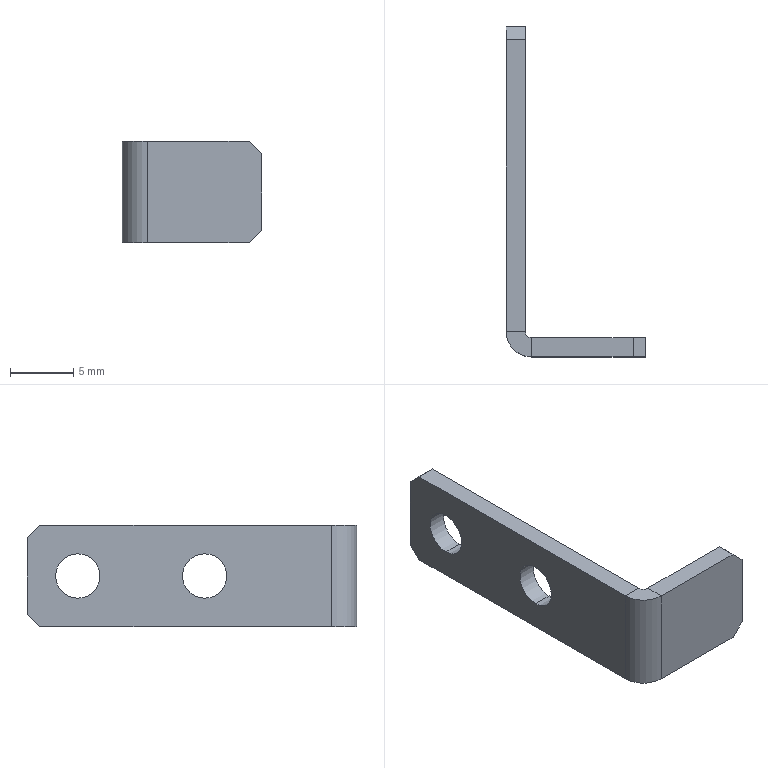Part | SolidWorks | features Chamfer 1, FlatPattern 1, HoleWzd 1, SMBaseFlange 1, SheetMetal 1 | 1 solid | 22 faces | box 11 x 26 x 8 mm | volume 387.699 mm3 | plane 16 | cylinder 6 | commonest cylinder face diameters 3.5 x4 1 x1 4 x1
STEP:
#1=CARTESIAN_POINT('',(1.5,22.,5.75));
#2=VERTEX_POINT('',#1);
#3=CARTESIAN_POINT('',(1.5,22.,2.25));
#4=VERTEX_POINT('',#3);
#5=CARTESIAN_POINT('',(1.5,22.,4.));
#6=DIRECTION('',(1.,0.,0.));
#7=DIRECTION('',(0.,1.,0.));
#8=AXIS2_PLACEMENT_3D('',#5,#6,#7);
#9=CIRCLE('',#8,1.75);
#10=EDGE_CURVE('',#2,#4,#9,.T.);
#11=ORIENTED_EDGE('',*,*,#10,.T.);
#12=CARTESIAN_POINT('',(0.,22.,2.25));
#13=VERTEX_POINT('',#12);
#14=CARTESIAN_POINT('',(0.,22.,2.25));
#15=DIRECTION('',(-1.,0.,0.));
#16=VECTOR('',#15,1000.);
#17=LINE('',#14,#16);
#18=EDGE_CURVE('',#4,#13,#17,.T.);
#19=ORIENTED_EDGE('',*,*,#18,.T.);
#20=CARTESIAN_POINT('',(0.,22.,5.75));
#21=VERTEX_POINT('',#20);
#22=CARTESIAN_POINT('',(0.,22.,4.));
#23=DIRECTION('',(-1.,0.,0.));
#24=DIRECTION('',(0.,0.,1.));
#25=AXIS2_PLACEMENT_3D('',#22,#23,#24);
#26=CIRCLE('',#25,1.75);
#27=EDGE_CURVE('',#13,#21,#26,.T.);
#28=ORIENTED_EDGE('',*,*,#27,.T.);
#29=CARTESIAN_POINT('',(0.,22.,5.75));
#30=DIRECTION('',(-1.,0.,0.));
#31=VECTOR('',#30,1000.);
#32=LINE('',#29,#31);
#33=EDGE_CURVE('',#2,#21,#32,.T.);
#34=ORIENTED_EDGE('',*,*,#33,.F.);
#35=EDGE_LOOP('',(#11,#19,#28,#34));
#36=FACE_OUTER_BOUND('',#35,.T.);
#37=CARTESIAN_POINT('',(0.,22.,4.));
#38=DIRECTION('',(-1.,0.,0.));
#39=DIRECTION('',(0.,0.,1.));
#40=AXIS2_PLACEMENT_3D('',#37,#38,#39);
#41=CYLINDRICAL_SURFACE('',#40,1.75);
#42=ADVANCED_FACE('',(#36),#41,.F.);
#43=CARTESIAN_POINT('',(1.5,12.,5.75));
#44=VERTEX_POINT('',#43);
#45=CARTESIAN_POINT('',(1.5,12.,2.25));
#46=VERTEX_POINT('',#45);
#47=CARTESIAN_POINT('',(1.5,12.,4.));
#48=DIRECTION('',(1.,0.,0.));
#49=DIRECTION('',(0.,1.,0.));
#50=AXIS2_PLACEMENT_3D('',#47,#48,#49);
#51=CIRCLE('',#50,1.75);
#52=EDGE_CURVE('',#44,#46,#51,.T.);
#53=ORIENTED_EDGE('',*,*,#52,.T.);
#54=CARTESIAN_POINT('',(0.,12.,2.25));
#55=VERTEX_POINT('',#54);
#56=CARTESIAN_POINT('',(0.,12.,2.25));
#57=DIRECTION('',(-1.,0.,0.));
#58=VECTOR('',#57,1000.);
#59=LINE('',#56,#58);
#60=EDGE_CURVE('',#46,#55,#59,.T.);
#61=ORIENTED_EDGE('',*,*,#60,.T.);
#62=CARTESIAN_POINT('',(0.,12.,5.75));
#63=VERTEX_POINT('',#62);
#64=CARTESIAN_POINT('',(0.,12.,4.));
#65=DIRECTION('',(-1.,0.,0.));
#66=DIRECTION('',(0.,0.,1.));
#67=AXIS2_PLACEMENT_3D('',#64,#65,#66);
#68=CIRCLE('',#67,1.75);
#69=EDGE_CURVE('',#55,#63,#68,.T.);
#70=ORIENTED_EDGE('',*,*,#69,.T.);
#71=CARTESIAN_POINT('',(0.,12.,5.75));
#72=DIRECTION('',(-1.,0.,0.));
#73=VECTOR('',#72,1000.);
#74=LINE('',#71,#73);
#75=EDGE_CURVE('',#44,#63,#74,.T.);
#76=ORIENTED_EDGE('',*,*,#75,.F.);
#77=EDGE_LOOP('',(#53,#61,#70,#76));
#78=FACE_OUTER_BOUND('',#77,.T.);
#79=CARTESIAN_POINT('',(0.,12.,4.));
#80=DIRECTION('',(-1.,0.,0.));
#81=DIRECTION('',(0.,0.,1.));
#82=AXIS2_PLACEMENT_3D('',#79,#80,#81);
#83=CYLINDRICAL_SURFACE('',#82,1.75);
#84=ADVANCED_FACE('',(#78),#83,.F.);
#85=CARTESIAN_POINT('',(0.,2.,8.));
#86=VERTEX_POINT('',#85);
#87=CARTESIAN_POINT('',(1.5,2.,8.));
#88=VERTEX_POINT('',#87);
#89=CARTESIAN_POINT('',(0.,2.,8.));
#90=DIRECTION('',(1.,0.,0.));
#91=VECTOR('',#90,1000.);
#92=LINE('',#89,#91);
#93=EDGE_CURVE('',#86,#88,#92,.T.);
#94=ORIENTED_EDGE('',*,*,#93,.F.);
#95=CARTESIAN_POINT('',(2.,0.,8.));
#96=VERTEX_POINT('',#95);
#97=CARTESIAN_POINT('',(2.,2.,8.));
#98=DIRECTION('',(0.,0.,1.));
#99=DIRECTION('',(-1.,0.,0.));
#100=AXIS2_PLACEMENT_3D('',#97,#98,#99);
#101=CIRCLE('',#100,2.);
#102=EDGE_CURVE('',#86,#96,#101,.T.);
#103=ORIENTED_EDGE('',*,*,#102,.T.);
#104=CARTESIAN_POINT('',(2.,1.5,8.));
#105=VERTEX_POINT('',#104);
#106=CARTESIAN_POINT('',(2.,1.5,8.));
#107=DIRECTION('',(0.,-1.,0.));
#108=VECTOR('',#107,1000.);
#109=LINE('',#106,#108);
#110=EDGE_CURVE('',#105,#96,#109,.T.);
#111=ORIENTED_EDGE('',*,*,#110,.F.);
#112=CARTESIAN_POINT('',(2.,2.,8.));
#113=DIRECTION('',(0.,0.,1.));
#114=DIRECTION('',(1.,0.,0.));
#115=AXIS2_PLACEMENT_3D('',#112,#113,#114);
#116=CIRCLE('',#115,0.5);
#117=EDGE_CURVE('',#88,#105,#116,.T.);
#118=ORIENTED_EDGE('',*,*,#117,.F.);
#119=EDGE_LOOP('',(#94,#103,#111,#118));
#120=FACE_OUTER_BOUND('',#119,.T.);
#121=CARTESIAN_POINT('',(0.,2.,8.));
#122=DIRECTION('',(0.,0.,1.));
#123=DIRECTION('',(1.,0.,0.));
#124=AXIS2_PLACEMENT_3D('',#121,#122,#123);
#125=PLANE('',#124);
#126=ADVANCED_FACE('',(#120),#125,.T.);
#127=CARTESIAN_POINT('',(1.5,25.,8.));
#128=VERTEX_POINT('',#127);
#129=CARTESIAN_POINT('',(1.5,26.,8.));
#130=DIRECTION('',(0.,-1.,0.));
#131=VECTOR('',#130,1000.);
#132=LINE('',#129,#131);
#133=EDGE_CURVE('',#128,#88,#132,.T.);
#134=ORIENTED_EDGE('',*,*,#133,.F.);
#135=CARTESIAN_POINT('',(0.,25.,8.));
#136=VERTEX_POINT('',#135);
#137=CARTESIAN_POINT('',(2.,25.,8.));
#138=DIRECTION('',(-1.,0.,0.));
#139=VECTOR('',#138,1000.);
#140=LINE('',#137,#139);
#141=EDGE_CURVE('',#128,#136,#140,.T.);
#142=ORIENTED_EDGE('',*,*,#141,.T.);
#143=CARTESIAN_POINT('',(0.,26.,8.));
#144=DIRECTION('',(0.,-1.,0.));
#145=VECTOR('',#144,1000.);
#146=LINE('',#143,#145);
#147=EDGE_CURVE('',#136,#86,#146,.T.);
#148=ORIENTED_EDGE('',*,*,#147,.T.);
#149=ORIENTED_EDGE('',*,*,#93,.T.);
#150=EDGE_LOOP('',(#134,#142,#148,#149));
#151=FACE_OUTER_BOUND('',#150,.T.);
#152=CARTESIAN_POINT('',(2.,1.5,8.));
#153=DIRECTION('',(0.,0.,1.));
#154=DIRECTION('',(1.,0.,0.));
#155=AXIS2_PLACEMENT_3D('',#152,#153,#154);
#156=PLANE('',#155);
#157=ADVANCED_FACE('',(#151),#156,.T.);
#158=CARTESIAN_POINT('',(2.,0.,0.));
#159=VERTEX_POINT('',#158);
#160=CARTESIAN_POINT('',(2.,1.5,0.));
#161=VERTEX_POINT('',#160);
#162=CARTESIAN_POINT('',(2.,0.,0.));
#163=DIRECTION('',(0.,1.,0.));
#164=VECTOR('',#163,1000.);
#165=LINE('',#162,#164);
#166=EDGE_CURVE('',#159,#161,#165,.T.);
#167=ORIENTED_EDGE('',*,*,#166,.F.);
#168=CARTESIAN_POINT('',(0.,2.,0.));
#169=VERTEX_POINT('',#168);
#170=CARTESIAN_POINT('',(2.,2.,0.));
#171=DIRECTION('',(0.,0.,1.));
#172=DIRECTION('',(-1.,0.,0.));
#173=AXIS2_PLACEMENT_3D('',#170,#171,#172);
#174=CIRCLE('',#173,2.);
#175=EDGE_CURVE('',#169,#159,#174,.T.);
#176=ORIENTED_EDGE('',*,*,#175,.F.);
#177=CARTESIAN_POINT('',(1.5,2.,0.));
#178=VERTEX_POINT('',#177);
#179=CARTESIAN_POINT('',(1.5,2.,0.));
#180=DIRECTION('',(-1.,0.,0.));
#181=VECTOR('',#180,1000.);
#182=LINE('',#179,#181);
#183=EDGE_CURVE('',#178,#169,#182,.T.);
#184=ORIENTED_EDGE('',*,*,#183,.F.);
#185=CARTESIAN_POINT('',(2.,2.,0.));
#186=DIRECTION('',(0.,0.,1.));
#187=DIRECTION('',(1.,0.,0.));
#188=AXIS2_PLACEMENT_3D('',#185,#186,#187);
#189=CIRCLE('',#188,0.5);
#190=EDGE_CURVE('',#178,#161,#189,.T.);
#191=ORIENTED_EDGE('',*,*,#190,.T.);
#192=EDGE_LOOP('',(#167,#176,#184,#191));
#193=FACE_OUTER_BOUND('',#192,.T.);
#194=CARTESIAN_POINT('',(2.,0.,0.));
#195=DIRECTION('',(0.,0.,-1.));
#196=DIRECTION('',(-1.,0.,0.));
#197=AXIS2_PLACEMENT_3D('',#194,#195,#196);
#198=PLANE('',#197);
#199=ADVANCED_FACE('',(#193),#198,.T.);
#200=CARTESIAN_POINT('',(10.,1.5,0.));
#201=VERTEX_POINT('',#200);
#202=CARTESIAN_POINT('',(0.,1.5,0.));
#203=DIRECTION('',(1.,0.,0.));
#204=VECTOR('',#203,1000.);
#205=LINE('',#202,#204);
#206=EDGE_CURVE('',#161,#201,#205,.T.);
#207=ORIENTED_EDGE('',*,*,#206,.T.);
#208=CARTESIAN_POINT('',(10.,0.,0.));
#209=VERTEX_POINT('',#208);
#210=CARTESIAN_POINT('',(10.,2.,0.));
#211=DIRECTION('',(0.,-1.,0.));
#212=VECTOR('',#211,1000.);
#213=LINE('',#210,#212);
#214=EDGE_CURVE('',#201,#209,#213,.T.);
#215=ORIENTED_EDGE('',*,*,#214,.T.);
#216=CARTESIAN_POINT('',(0.,0.,0.));
#217=DIRECTION('',(1.,0.,0.));
#218=VECTOR('',#217,1000.);
#219=LINE('',#216,#218);
#220=EDGE_CURVE('',#159,#209,#219,.T.);
#221=ORIENTED_EDGE('',*,*,#220,.F.);
#222=ORIENTED_EDGE('',*,*,#166,.T.);
#223=EDGE_LOOP('',(#207,#215,#221,#222));
#224=FACE_OUTER_BOUND('',#223,.T.);
#225=CARTESIAN_POINT('',(1.5,2.,0.));
#226=DIRECTION('',(0.,0.,-1.));
#227=DIRECTION('',(-1.,0.,0.));
#228=AXIS2_PLACEMENT_3D('',#225,#226,#227);
#229=PLANE('',#228);
#230=ADVANCED_FACE('',(#224),#229,.T.);
#231=ORIENTED_EDGE('',*,*,#220,.T.);
#232=CARTESIAN_POINT('',(11.,0.,1.));
#233=VERTEX_POINT('',#232);
#234=CARTESIAN_POINT('',(10.,0.,0.));
#235=DIRECTION('',(0.7071,0.,0.7071));
#236=VECTOR('',#235,1000.);
#237=LINE('',#234,#236);
#238=EDGE_CURVE('',#209,#233,#237,.T.);
#239=ORIENTED_EDGE('',*,*,#238,.T.);
#240=CARTESIAN_POINT('',(11.,0.,7.));
#241=VERTEX_POINT('',#240);
#242=CARTESIAN_POINT('',(11.,0.,8.));
#243=DIRECTION('',(0.,0.,-1.));
#244=VECTOR('',#243,1000.);
#245=LINE('',#242,#244);
#246=EDGE_CURVE('',#241,#233,#245,.T.);
#247=ORIENTED_EDGE('',*,*,#246,.F.);
#248=CARTESIAN_POINT('',(10.,0.,8.));
#249=VERTEX_POINT('',#248);
#250=CARTESIAN_POINT('',(11.,0.,7.));
#251=DIRECTION('',(-0.7071,0.,0.7071));
#252=VECTOR('',#251,1000.);
#253=LINE('',#250,#252);
#254=EDGE_CURVE('',#241,#249,#253,.T.);
#255=ORIENTED_EDGE('',*,*,#254,.T.);
#256=CARTESIAN_POINT('',(0.,0.,8.));
#257=DIRECTION('',(1.,0.,0.));
#258=VECTOR('',#257,1000.);
#259=LINE('',#256,#258);
#260=EDGE_CURVE('',#96,#249,#259,.T.);
#261=ORIENTED_EDGE('',*,*,#260,.F.);
#262=CARTESIAN_POINT('',(2.,0.,8.));
#263=DIRECTION('',(0.,0.,-1.));
#264=VECTOR('',#263,1000.);
#265=LINE('',#262,#264);
#266=EDGE_CURVE('',#96,#159,#265,.T.);
#267=ORIENTED_EDGE('',*,*,#266,.T.);
#268=EDGE_LOOP('',(#231,#239,#247,#255,#261,#267));
#269=FACE_OUTER_BOUND('',#268,.T.);
#270=CARTESIAN_POINT('',(0.,0.,8.));
#271=DIRECTION('',(0.,1.,0.));
#272=DIRECTION('',(0.,0.,1.));
#273=AXIS2_PLACEMENT_3D('',#270,#271,#272);
#274=PLANE('',#273);
#275=ADVANCED_FACE('',(#269),#274,.F.);
#276=ORIENTED_EDGE('',*,*,#246,.T.);
#277=CARTESIAN_POINT('',(11.,1.5,1.));
#278=VERTEX_POINT('',#277);
#279=CARTESIAN_POINT('',(11.,1.5,1.));
#280=DIRECTION('',(0.,1.,0.));
#281=VECTOR('',#280,1000.);
#282=LINE('',#279,#281);
#283=EDGE_CURVE('',#233,#278,#282,.T.);
#284=ORIENTED_EDGE('',*,*,#283,.T.);
#285=CARTESIAN_POINT('',(11.,1.5,7.));
#286=VERTEX_POINT('',#285);
#287=CARTESIAN_POINT('',(11.,1.5,8.));
#288=DIRECTION('',(0.,0.,-1.));
#289=VECTOR('',#288,1000.);
#290=LINE('',#287,#289);
#291=EDGE_CURVE('',#286,#278,#290,.T.);
#292=ORIENTED_EDGE('',*,*,#291,.F.);
#293=CARTESIAN_POINT('',(11.,1.5,7.));
#294=DIRECTION('',(0.,-1.,0.));
#295=VECTOR('',#294,1000.);
#296=LINE('',#293,#295);
#297=EDGE_CURVE('',#286,#241,#296,.T.);
#298=ORIENTED_EDGE('',*,*,#297,.T.);
#299=EDGE_LOOP('',(#276,#284,#292,#298));
#300=FACE_OUTER_BOUND('',#299,.T.);
#301=CARTESIAN_POINT('',(11.,1.5,8.));
#302=DIRECTION('',(1.,0.,0.));
#303=DIRECTION('',(0.,0.,-1.));
#304=AXIS2_PLACEMENT_3D('',#301,#302,#303);
#305=PLANE('',#304);
#306=ADVANCED_FACE('',(#300),#305,.T.);
#307=ORIENTED_EDGE('',*,*,#291,.T.);
#308=CARTESIAN_POINT('',(9.,1.5,-1.));
#309=DIRECTION('',(-0.7071,0.,-0.7071));
#310=VECTOR('',#309,1000.);
#311=LINE('',#308,#310);
#312=EDGE_CURVE('',#278,#201,#311,.T.);
#313=ORIENTED_EDGE('',*,*,#312,.T.);
#314=ORIENTED_EDGE('',*,*,#206,.F.);
#315=CARTESIAN_POINT('',(2.,1.5,8.));
#316=DIRECTION('',(0.,0.,-1.));
#317=VECTOR('',#316,1000.);
#318=LINE('',#315,#317);
#319=EDGE_CURVE('',#105,#161,#318,.T.);
#320=ORIENTED_EDGE('',*,*,#319,.F.);
#321=CARTESIAN_POINT('',(10.,1.5,8.));
#322=VERTEX_POINT('',#321);
#323=CARTESIAN_POINT('',(0.,1.5,8.));
#324=DIRECTION('',(1.,0.,0.));
#325=VECTOR('',#324,1000.);
#326=LINE('',#323,#325);
#327=EDGE_CURVE('',#105,#322,#326,.T.);
#328=ORIENTED_EDGE('',*,*,#327,.T.);
#329=CARTESIAN_POINT('',(5.,1.5,13.));
#330=DIRECTION('',(0.7071,0.,-0.7071));
#331=VECTOR('',#330,1000.);
#332=LINE('',#329,#331);
#333=EDGE_CURVE('',#322,#286,#332,.T.);
#334=ORIENTED_EDGE('',*,*,#333,.T.);
#335=EDGE_LOOP('',(#307,#313,#314,#320,#328,#334));
#336=FACE_OUTER_BOUND('',#335,.T.);
#337=CARTESIAN_POINT('',(0.,1.5,8.));
#338=DIRECTION('',(0.,1.,0.));
#339=DIRECTION('',(0.,0.,1.));
#340=AXIS2_PLACEMENT_3D('',#337,#338,#339);
#341=PLANE('',#340);
#342=ADVANCED_FACE('',(#336),#341,.T.);
#343=ORIENTED_EDGE('',*,*,#190,.F.);
#344=CARTESIAN_POINT('',(1.5,2.,8.));
#345=DIRECTION('',(0.,0.,-1.));
#346=VECTOR('',#345,1000.);
#347=LINE('',#344,#346);
#348=EDGE_CURVE('',#88,#178,#347,.T.);
#349=ORIENTED_EDGE('',*,*,#348,.F.);
#350=ORIENTED_EDGE('',*,*,#117,.T.);
#351=ORIENTED_EDGE('',*,*,#319,.T.);
#352=EDGE_LOOP('',(#343,#349,#350,#351));
#353=FACE_OUTER_BOUND('',#352,.T.);
#354=CARTESIAN_POINT('',(2.,2.,8.));
#355=DIRECTION('',(0.,0.,-1.));
#356=DIRECTION('',(-1.,0.,0.));
#357=AXIS2_PLACEMENT_3D('',#354,#355,#356);
#358=CYLINDRICAL_SURFACE('',#357,0.5);
#359=ADVANCED_FACE('',(#353),#358,.F.);
#360=ORIENTED_EDGE('',*,*,#10,.F.);
#361=CARTESIAN_POINT('',(1.5,22.,4.));
#362=DIRECTION('',(1.,0.,0.));
#363=DIRECTION('',(0.,1.,0.));
#364=AXIS2_PLACEMENT_3D('',#361,#362,#363);
#365=CIRCLE('',#364,1.75);
#366=EDGE_CURVE('',#4,#2,#365,.T.);
#367=ORIENTED_EDGE('',*,*,#366,.F.);
#368=EDGE_LOOP('',(#360,#367));
#369=FACE_BOUND('',#368,.T.);
#370=ORIENTED_EDGE('',*,*,#52,.F.);
#371=CARTESIAN_POINT('',(1.5,12.,4.));
#372=DIRECTION('',(1.,0.,0.));
#373=DIRECTION('',(0.,1.,0.));
#374=AXIS2_PLACEMENT_3D('',#371,#372,#373);
#375=CIRCLE('',#374,1.75);
#376=EDGE_CURVE('',#46,#44,#375,.T.);
#377=ORIENTED_EDGE('',*,*,#376,.F.);
#378=EDGE_LOOP('',(#370,#377));
#379=FACE_BOUND('',#378,.T.);
#380=CARTESIAN_POINT('',(1.5,25.,0.));
#381=VERTEX_POINT('',#380);
#382=CARTESIAN_POINT('',(1.5,26.,0.));
#383=DIRECTION('',(0.,-1.,0.));
#384=VECTOR('',#383,1000.);
#385=LINE('',#382,#384);
#386=EDGE_CURVE('',#381,#178,#385,.T.);
#387=ORIENTED_EDGE('',*,*,#386,.F.);
#388=CARTESIAN_POINT('',(1.5,26.,1.));
#389=VERTEX_POINT('',#388);
#390=CARTESIAN_POINT('',(1.5,29.5,4.5));
#391=DIRECTION('',(0.,0.7071,0.7071));
#392=VECTOR('',#391,1000.);
#393=LINE('',#390,#392);
#394=EDGE_CURVE('',#381,#389,#393,.T.);
#395=ORIENTED_EDGE('',*,*,#394,.T.);
#396=CARTESIAN_POINT('',(1.5,26.,7.));
#397=VERTEX_POINT('',#396);
#398=CARTESIAN_POINT('',(1.5,26.,8.));
#399=DIRECTION('',(0.,0.,-1.));
#400=VECTOR('',#399,1000.);
#401=LINE('',#398,#400);
#402=EDGE_CURVE('',#397,#389,#401,.T.);
#403=ORIENTED_EDGE('',*,*,#402,.F.);
#404=CARTESIAN_POINT('',(1.5,25.5,7.5));
#405=DIRECTION('',(0.,-0.7071,0.7071));
#406=VECTOR('',#405,1000.);
#407=LINE('',#404,#406);
#408=EDGE_CURVE('',#397,#128,#407,.T.);
#409=ORIENTED_EDGE('',*,*,#408,.T.);
#410=ORIENTED_EDGE('',*,*,#133,.T.);
#411=ORIENTED_EDGE('',*,*,#348,.T.);
#412=EDGE_LOOP('',(#387,#395,#403,#409,#410,#411));
#413=FACE_OUTER_BOUND('',#412,.T.);
#414=CARTESIAN_POINT('',(1.5,26.,8.));
#415=DIRECTION('',(1.,0.,0.));
#416=DIRECTION('',(0.,1.,0.));
#417=AXIS2_PLACEMENT_3D('',#414,#415,#416);
#418=PLANE('',#417);
#419=ADVANCED_FACE('',(#369,#379,#413),#418,.T.);
#420=ORIENTED_EDGE('',*,*,#402,.T.);
#421=CARTESIAN_POINT('',(0.,26.,1.));
#422=VERTEX_POINT('',#421);
#423=CARTESIAN_POINT('',(0.,26.,1.));
#424=DIRECTION('',(-1.,0.,0.));
#425=VECTOR('',#424,1000.);
#426=LINE('',#423,#425);
#427=EDGE_CURVE('',#389,#422,#426,.T.);
#428=ORIENTED_EDGE('',*,*,#427,.T.);
#429=CARTESIAN_POINT('',(0.,26.,7.));
#430=VERTEX_POINT('',#429);
#431=CARTESIAN_POINT('',(0.,26.,8.));
#432=DIRECTION('',(0.,0.,-1.));
#433=VECTOR('',#432,1000.);
#434=LINE('',#431,#433);
#435=EDGE_CURVE('',#430,#422,#434,.T.);
#436=ORIENTED_EDGE('',*,*,#435,.F.);
#437=CARTESIAN_POINT('',(0.,26.,7.));
#438=DIRECTION('',(1.,0.,0.));
#439=VECTOR('',#438,1000.);
#440=LINE('',#437,#439);
#441=EDGE_CURVE('',#430,#397,#440,.T.);
#442=ORIENTED_EDGE('',*,*,#441,.T.);
#443=EDGE_LOOP('',(#420,#428,#436,#442));
#444=FACE_OUTER_BOUND('',#443,.T.);
#445=CARTESIAN_POINT('',(0.,26.,8.));
#446=DIRECTION('',(0.,1.,0.));
#447=DIRECTION('',(0.,0.,1.));
#448=AXIS2_PLACEMENT_3D('',#445,#446,#447);
#449=PLANE('',#448);
#450=ADVANCED_FACE('',(#444),#449,.T.);
#451=CARTESIAN_POINT('',(0.,22.,4.));
#452=DIRECTION('',(-1.,0.,0.));
#453=DIRECTION('',(0.,0.,1.));
#454=AXIS2_PLACEMENT_3D('',#451,#452,#453);
#455=CIRCLE('',#454,1.75);
#456=EDGE_CURVE('',#21,#13,#455,.T.);
#457=ORIENTED_EDGE('',*,*,#456,.F.);
#458=ORIENTED_EDGE('',*,*,#27,.F.);
#459=EDGE_LOOP('',(#457,#458));
#460=FACE_BOUND('',#459,.T.);
#461=CARTESIAN_POINT('',(0.,12.,4.));
#462=DIRECTION('',(-1.,0.,0.));
#463=DIRECTION('',(0.,0.,1.));
#464=AXIS2_PLACEMENT_3D('',#461,#462,#463);
#465=CIRCLE('',#464,1.75);
#466=EDGE_CURVE('',#63,#55,#465,.T.);
#467=ORIENTED_EDGE('',*,*,#466,.F.);
#468=ORIENTED_EDGE('',*,*,#69,.F.);
#469=EDGE_LOOP('',(#467,#468));
#470=FACE_BOUND('',#469,.T.);
#471=ORIENTED_EDGE('',*,*,#435,.T.);
#472=CARTESIAN_POINT('',(0.,25.,0.));
#473=VERTEX_POINT('',#472);
#474=CARTESIAN_POINT('',(0.,25.,0.));
#475=DIRECTION('',(0.,-0.7071,-0.7071));
#476=VECTOR('',#475,1000.);
#477=LINE('',#474,#476);
#478=EDGE_CURVE('',#422,#473,#477,.T.);
#479=ORIENTED_EDGE('',*,*,#478,.T.);
#480=CARTESIAN_POINT('',(0.,26.,0.));
#481=DIRECTION('',(0.,-1.,0.));
#482=VECTOR('',#481,1000.);
#483=LINE('',#480,#482);
#484=EDGE_CURVE('',#473,#169,#483,.T.);
#485=ORIENTED_EDGE('',*,*,#484,.T.);
#486=CARTESIAN_POINT('',(0.,2.,8.));
#487=DIRECTION('',(0.,0.,-1.));
#488=VECTOR('',#487,1000.);
#489=LINE('',#486,#488);
#490=EDGE_CURVE('',#86,#169,#489,.T.);
#491=ORIENTED_EDGE('',*,*,#490,.F.);
#492=ORIENTED_EDGE('',*,*,#147,.F.);
#493=CARTESIAN_POINT('',(0.,26.,7.));
#494=DIRECTION('',(0.,0.7071,-0.7071));
#495=VECTOR('',#494,1000.);
#496=LINE('',#493,#495);
#497=EDGE_CURVE('',#136,#430,#496,.T.);
#498=ORIENTED_EDGE('',*,*,#497,.T.);
#499=EDGE_LOOP('',(#471,#479,#485,#491,#492,#498));
#500=FACE_OUTER_BOUND('',#499,.T.);
#501=CARTESIAN_POINT('',(0.,26.,8.));
#502=DIRECTION('',(1.,0.,0.));
#503=DIRECTION('',(0.,1.,0.));
#504=AXIS2_PLACEMENT_3D('',#501,#502,#503);
#505=PLANE('',#504);
#506=ADVANCED_FACE('',(#460,#470,#500),#505,.F.);
#507=ORIENTED_EDGE('',*,*,#175,.T.);
#508=ORIENTED_EDGE('',*,*,#266,.F.);
#509=ORIENTED_EDGE('',*,*,#102,.F.);
#510=ORIENTED_EDGE('',*,*,#490,.T.);
#511=EDGE_LOOP('',(#507,#508,#509,#510));
#512=FACE_OUTER_BOUND('',#511,.T.);
#513=CARTESIAN_POINT('',(2.,2.,8.));
#514=DIRECTION('',(0.,0.,-1.));
#515=DIRECTION('',(-1.,0.,0.));
#516=AXIS2_PLACEMENT_3D('',#513,#514,#515);
#517=CYLINDRICAL_SURFACE('',#516,2.);
#518=ADVANCED_FACE('',(#512),#517,.T.);
#519=ORIENTED_EDGE('',*,*,#260,.T.);
#520=CARTESIAN_POINT('',(10.,2.,8.));
#521=DIRECTION('',(0.,1.,0.));
#522=VECTOR('',#521,1000.);
#523=LINE('',#520,#522);
#524=EDGE_CURVE('',#249,#322,#523,.T.);
#525=ORIENTED_EDGE('',*,*,#524,.T.);
#526=ORIENTED_EDGE('',*,*,#327,.F.);
#527=ORIENTED_EDGE('',*,*,#110,.T.);
#528=EDGE_LOOP('',(#519,#525,#526,#527));
#529=FACE_OUTER_BOUND('',#528,.T.);
#530=CARTESIAN_POINT('',(2.,2.,8.));
#531=DIRECTION('',(0.,0.,1.));
#532=DIRECTION('',(1.,0.,0.));
#533=AXIS2_PLACEMENT_3D('',#530,#531,#532);
#534=PLANE('',#533);
#535=ADVANCED_FACE('',(#529),#534,.T.);
#536=ORIENTED_EDGE('',*,*,#484,.F.);
#537=CARTESIAN_POINT('',(1.5,25.,0.));
#538=DIRECTION('',(1.,0.,0.));
#539=VECTOR('',#538,1000.);
#540=LINE('',#537,#539);
#541=EDGE_CURVE('',#473,#381,#540,.T.);
#542=ORIENTED_EDGE('',*,*,#541,.T.);
#543=ORIENTED_EDGE('',*,*,#386,.T.);
#544=ORIENTED_EDGE('',*,*,#183,.T.);
#545=EDGE_LOOP('',(#536,#542,#543,#544));
#546=FACE_OUTER_BOUND('',#545,.T.);
#547=CARTESIAN_POINT('',(2.,2.,0.));
#548=DIRECTION('',(0.,0.,1.));
#549=DIRECTION('',(1.,0.,0.));
#550=AXIS2_PLACEMENT_3D('',#547,#548,#549);
#551=PLANE('',#550);
#552=ADVANCED_FACE('',(#546),#551,.F.);
#553=ORIENTED_EDGE('',*,*,#60,.F.);
#554=ORIENTED_EDGE('',*,*,#376,.T.);
#555=ORIENTED_EDGE('',*,*,#75,.T.);
#556=ORIENTED_EDGE('',*,*,#466,.T.);
#557=EDGE_LOOP('',(#553,#554,#555,#556));
#558=FACE_OUTER_BOUND('',#557,.T.);
#559=CARTESIAN_POINT('',(0.,12.,4.));
#560=DIRECTION('',(-1.,0.,0.));
#561=DIRECTION('',(0.,0.,1.));
#562=AXIS2_PLACEMENT_3D('',#559,#560,#561);
#563=CYLINDRICAL_SURFACE('',#562,1.75);
#564=ADVANCED_FACE('',(#558),#563,.F.);
#565=ORIENTED_EDGE('',*,*,#18,.F.);
#566=ORIENTED_EDGE('',*,*,#366,.T.);
#567=ORIENTED_EDGE('',*,*,#33,.T.);
#568=ORIENTED_EDGE('',*,*,#456,.T.);
#569=EDGE_LOOP('',(#565,#566,#567,#568));
#570=FACE_OUTER_BOUND('',#569,.T.);
#571=CARTESIAN_POINT('',(0.,22.,4.));
#572=DIRECTION('',(-1.,0.,0.));
#573=DIRECTION('',(0.,0.,1.));
#574=AXIS2_PLACEMENT_3D('',#571,#572,#573);
#575=CYLINDRICAL_SURFACE('',#574,1.75);
#576=ADVANCED_FACE('',(#570),#575,.F.);
#577=ORIENTED_EDGE('',*,*,#312,.F.);
#578=ORIENTED_EDGE('',*,*,#283,.F.);
#579=ORIENTED_EDGE('',*,*,#238,.F.);
#580=ORIENTED_EDGE('',*,*,#214,.F.);
#581=EDGE_LOOP('',(#577,#578,#579,#580));
#582=FACE_OUTER_BOUND('',#581,.T.);
#583=CARTESIAN_POINT('',(10.,2.,0.));
#584=DIRECTION('',(-0.7071,0.,0.7071));
#585=DIRECTION('',(0.,-1.,0.));
#586=AXIS2_PLACEMENT_3D('',#583,#584,#585);
#587=PLANE('',#586);
#588=ADVANCED_FACE('',(#582),#587,.F.);
#589=ORIENTED_EDGE('',*,*,#333,.F.);
#590=ORIENTED_EDGE('',*,*,#524,.F.);
#591=ORIENTED_EDGE('',*,*,#254,.F.);
#592=ORIENTED_EDGE('',*,*,#297,.F.);
#593=EDGE_LOOP('',(#589,#590,#591,#592));
#594=FACE_OUTER_BOUND('',#593,.T.);
#595=CARTESIAN_POINT('',(11.,1.5,7.));
#596=DIRECTION('',(-0.7071,0.,-0.7071));
#597=DIRECTION('',(0.,-1.,0.));
#598=AXIS2_PLACEMENT_3D('',#595,#596,#597);
#599=PLANE('',#598);
#600=ADVANCED_FACE('',(#594),#599,.F.);
#601=ORIENTED_EDGE('',*,*,#478,.F.);
#602=ORIENTED_EDGE('',*,*,#427,.F.);
#603=ORIENTED_EDGE('',*,*,#394,.F.);
#604=ORIENTED_EDGE('',*,*,#541,.F.);
#605=EDGE_LOOP('',(#601,#602,#603,#604));
#606=FACE_OUTER_BOUND('',#605,.T.);
#607=CARTESIAN_POINT('',(2.,25.,0.));
#608=DIRECTION('',(0.,0.7071,-0.7071));
#609=DIRECTION('',(-1.,0.,0.));
#610=AXIS2_PLACEMENT_3D('',#607,#608,#609);
#611=PLANE('',#610);
#612=ADVANCED_FACE('',(#606),#611,.T.);
#613=ORIENTED_EDGE('',*,*,#497,.F.);
#614=ORIENTED_EDGE('',*,*,#141,.F.);
#615=ORIENTED_EDGE('',*,*,#408,.F.);
#616=ORIENTED_EDGE('',*,*,#441,.F.);
#617=EDGE_LOOP('',(#613,#614,#615,#616));
#618=FACE_OUTER_BOUND('',#617,.T.);
#619=CARTESIAN_POINT('',(0.,26.,7.));
#620=DIRECTION('',(0.,-0.7071,-0.7071));
#621=DIRECTION('',(1.,0.,0.));
#622=AXIS2_PLACEMENT_3D('',#619,#620,#621);
#623=PLANE('',#622);
#624=ADVANCED_FACE('',(#618),#623,.F.);
#625=CLOSED_SHELL('',(#42,#84,#126,#157,#199,#230,#275,#306,#342,#359,#419,#450,#506,#518,#535,#552,#564,#576,#588,#600,#612,#624));
#626=MANIFOLD_SOLID_BREP('',#625);
#627=CARTESIAN_POINT('',(0.,0.,0.));
#628=DIRECTION('',(0.,0.,1.));
#629=DIRECTION('',(1.,0.,0.));
#630=AXIS2_PLACEMENT_3D('',#627,#628,#629);
#631=(LENGTH_UNIT()NAMED_UNIT(*)SI_UNIT(.MILLI.,.METRE.));
#632=UNCERTAINTY_MEASURE_WITH_UNIT(LENGTH_MEASURE(0.00001),#631,'','');
#633=(NAMED_UNIT(*)PLANE_ANGLE_UNIT()SI_UNIT($,.RADIAN.));
#634=(NAMED_UNIT(*)SI_UNIT($,.STERADIAN.)SOLID_ANGLE_UNIT());
#635=(GEOMETRIC_REPRESENTATION_CONTEXT(3)GLOBAL_UNCERTAINTY_ASSIGNED_CONTEXT((#632))GLOBAL_UNIT_ASSIGNED_CONTEXT((#631,#633,#634))REPRESENTATION_CONTEXT('',''));
#636=ADVANCED_BREP_SHAPE_REPRESENTATION('',(#626,#630),#635);